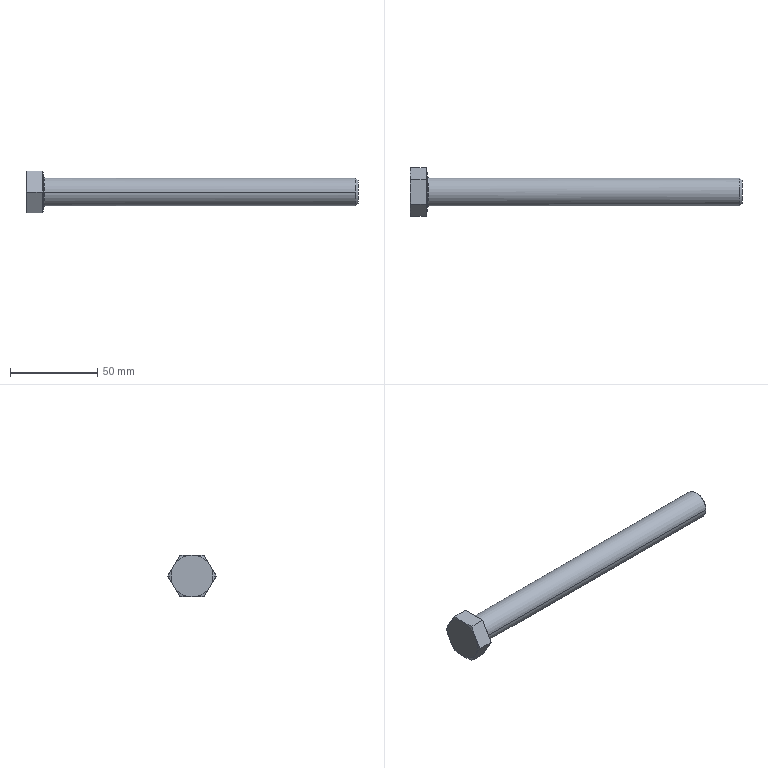Part | STEP file | HEX. HEAD-M16x180 | 1 solid | 28 faces | box 190 x 27.713 x 24 mm | volume 41063 mm3 | cone 12 | plane 10 | cylinder 4 | torus 2 | commonest cylinder face diameters 16 x2 22 x2